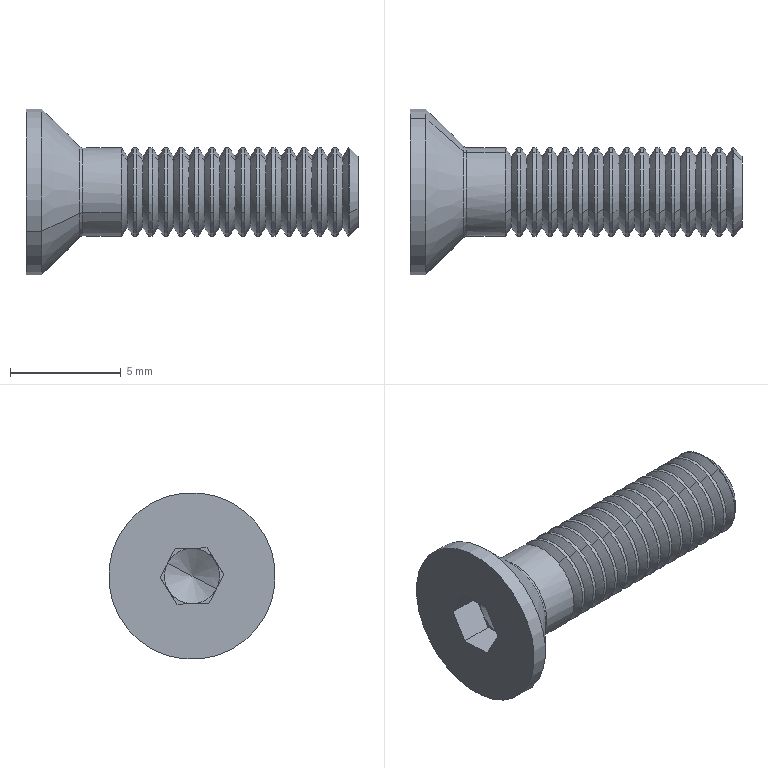Part | STEP file | Completa.sldasm-Part-62_Valor predeterminado | 1 solid | 116 faces | box 15 x 7.53 x 7.53 mm | volume 207.73 mm3 | cone 66 | cylinder 34 | plane 14 | torus 2 | commonest cylinder face diameters 4 x32 7.53 x2